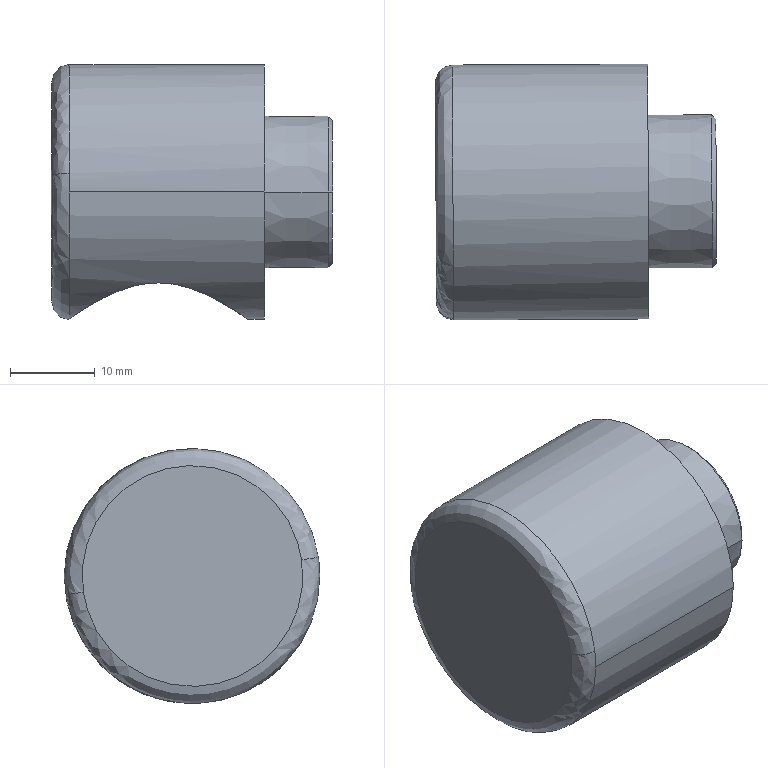Part | SolidWorks | features BaseBody 1 | 1 solid | 24 faces | box 33.093 x 30.1 x 30 mm | volume 10918 mm3 | cone 13 | spline 4 | cylinder 4 | plane 3 | commonest cylinder face diameters 16 x2 30 x2
STEP:
#1=CARTESIAN_POINT('',(688.091,25.759,6.001));
#2=VERTEX_POINT('',#1);
#3=CARTESIAN_POINT('',(687.979,51.477,2.182));
#4=VERTEX_POINT('',#3);
#5=CARTESIAN_POINT('',(688.091,25.759,6.001));
#6=CARTESIAN_POINT('',(688.107,21.94,-19.717));
#7=CARTESIAN_POINT('',(687.996,47.658,-23.536));
#8=CARTESIAN_POINT('',(687.979,51.477,2.182));
#9=(BOUNDED_CURVE()B_SPLINE_CURVE(3,(#5,#6,#7,#8),.UNSPECIFIED.,.F.,.F.)B_SPLINE_CURVE_WITH_KNOTS((4,4),(0.,1.),.UNSPECIFIED.)CURVE()GEOMETRIC_REPRESENTATION_ITEM()RATIONAL_B_SPLINE_CURVE((1.,0.3333,0.3333,1.))REPRESENTATION_ITEM(''));
#10=EDGE_CURVE('',#2,#4,#9,.T.);
#11=ORIENTED_EDGE('',*,*,#10,.T.);
#12=CARTESIAN_POINT('',(689.97,53.464,1.889));
#13=VERTEX_POINT('',#12);
#14=CARTESIAN_POINT('',(689.979,51.485,2.182));
#15=DIRECTION('',(0.0006392,-0.1469,-0.9892));
#16=DIRECTION('',(-0.004305,0.9891,-0.1469));
#17=AXIS2_PLACEMENT_3D('',#14,#15,#16);
#18=CIRCLE('',#17,2.);
#19=EDGE_CURVE('',#4,#13,#18,.T.);
#20=ORIENTED_EDGE('',*,*,#19,.T.);
#21=CARTESIAN_POINT('',(690.029,39.954,-10.849));
#22=VERTEX_POINT('',#21);
#23=CARTESIAN_POINT('',(690.035,38.626,4.092));
#24=DIRECTION('',(1.,0.004352,-0.000000001));
#25=DIRECTION('',(0.004352,-1.,0.));
#26=AXIS2_PLACEMENT_3D('',#23,#24,#25);
#27=CIRCLE('',#26,15.);
#28=EDGE_CURVE('',#22,#13,#27,.T.);
#29=ORIENTED_EDGE('',*,*,#28,.F.);
#30=CARTESIAN_POINT('',(690.041,37.299,-10.849));
#31=VERTEX_POINT('',#30);
#32=CARTESIAN_POINT('',(690.029,39.954,-10.849));
#33=CARTESIAN_POINT('',(689.974,39.511,-10.889));
#34=CARTESIAN_POINT('',(689.922,38.626,-10.924));
#35=CARTESIAN_POINT('',(689.982,37.741,-10.889));
#36=CARTESIAN_POINT('',(690.041,37.299,-10.849));
#37=B_SPLINE_CURVE_WITH_KNOTS('',3,(#32,#33,#34,#35,#36),.UNSPECIFIED.,.F.,.F.,(4,1,4),(0.,0.001328,0.002656),.UNSPECIFIED.);
#38=EDGE_CURVE('',#22,#31,#37,.T.);
#39=ORIENTED_EDGE('',*,*,#38,.T.);
#40=CARTESIAN_POINT('',(690.1,23.627,4.092));
#41=VERTEX_POINT('',#40);
#42=CARTESIAN_POINT('',(690.035,38.626,4.092));
#43=DIRECTION('',(1.,0.004352,-0.000000001));
#44=DIRECTION('',(0.004352,-1.,0.));
#45=AXIS2_PLACEMENT_3D('',#42,#43,#44);
#46=CIRCLE('',#45,15.);
#47=EDGE_CURVE('',#41,#31,#46,.T.);
#48=ORIENTED_EDGE('',*,*,#47,.F.);
#49=CARTESIAN_POINT('',(690.099,23.789,6.295));
#50=VERTEX_POINT('',#49);
#51=CARTESIAN_POINT('',(690.035,38.626,4.092));
#52=DIRECTION('',(1.,0.004352,-0.000000001));
#53=DIRECTION('',(0.004352,-1.,0.));
#54=AXIS2_PLACEMENT_3D('',#51,#52,#53);
#55=CIRCLE('',#54,15.);
#56=EDGE_CURVE('',#50,#41,#55,.T.);
#57=ORIENTED_EDGE('',*,*,#56,.F.);
#58=CARTESIAN_POINT('',(690.091,25.768,6.001));
#59=DIRECTION('',(-0.0006392,0.1469,0.9892));
#60=DIRECTION('',(0.004305,-0.9891,0.1469));
#61=AXIS2_PLACEMENT_3D('',#58,#59,#60);
#62=CIRCLE('',#61,2.);
#63=EDGE_CURVE('',#2,#50,#62,.T.);
#64=ORIENTED_EDGE('',*,*,#63,.F.);
#65=EDGE_LOOP('',(#11,#20,#29,#39,#48,#57,#64));
#66=FACE_OUTER_BOUND('',#65,.T.);
#67=CARTESIAN_POINT('',(687.979,51.477,2.182));
#68=CARTESIAN_POINT('',(687.996,47.658,-23.536));
#69=CARTESIAN_POINT('',(688.107,21.94,-19.717));
#70=CARTESIAN_POINT('',(688.091,25.759,6.001));
#71=CARTESIAN_POINT('',(687.974,52.636,2.01));
#72=CARTESIAN_POINT('',(687.992,48.473,-26.025));
#73=CARTESIAN_POINT('',(688.114,20.437,-21.863));
#74=CARTESIAN_POINT('',(688.096,24.6,6.173));
#75=CARTESIAN_POINT('',(688.799,53.459,1.889));
#76=CARTESIAN_POINT('',(688.818,49.053,-27.786));
#77=CARTESIAN_POINT('',(688.947,19.378,-23.38));
#78=CARTESIAN_POINT('',(688.928,23.784,6.295));
#79=CARTESIAN_POINT('',(689.97,53.464,1.889));
#80=CARTESIAN_POINT('',(689.989,49.058,-27.786));
#81=CARTESIAN_POINT('',(690.119,19.383,-23.38));
#82=CARTESIAN_POINT('',(690.099,23.789,6.295));
#83=(BOUNDED_SURFACE()B_SPLINE_SURFACE(3,3,((#67,#68,#69,#70),(#71,#72,#73,#74),(#75,#76,#77,#78),(#79,#80,#81,#82)),.UNSPECIFIED.,.F.,.F.,.F.)B_SPLINE_SURFACE_WITH_KNOTS((4,4),(4,4),(0.,1.),(0.,1.),.UNSPECIFIED.)GEOMETRIC_REPRESENTATION_ITEM()RATIONAL_B_SPLINE_SURFACE(((1.,0.3333,0.3333,1.),(0.8047,0.2682,0.2682,0.8047),(0.8047,0.2682,0.2682,0.8047),(1.,0.3333,0.3333,1.)))REPRESENTATION_ITEM('')SURFACE());
#84=ADVANCED_FACE('',(#66),#83,.T.);
#85=CARTESIAN_POINT('',(721.071,30.355,5.34));
#86=VERTEX_POINT('',#85);
#87=CARTESIAN_POINT('',(720.998,47.26,4.092));
#88=VERTEX_POINT('',#87);
#89=CARTESIAN_POINT('',(721.035,38.761,4.092));
#90=DIRECTION('',(-1.,-0.004352,0.000000001));
#91=DIRECTION('',(0.004305,-0.9891,0.1469));
#92=AXIS2_PLACEMENT_3D('',#89,#90,#91);
#93=CIRCLE('',#92,8.499);
#94=EDGE_CURVE('',#86,#88,#93,.T.);
#95=ORIENTED_EDGE('',*,*,#94,.F.);
#96=CARTESIAN_POINT('',(720.204,30.844,5.267));
#97=VERTEX_POINT('',#96);
#98=CARTESIAN_POINT('',(720.208,29.855,5.413));
#99=DIRECTION('',(-0.0006392,0.1469,0.9892));
#100=DIRECTION('',(0.004305,-0.9891,0.1469));
#101=AXIS2_PLACEMENT_3D('',#98,#99,#100);
#102=CIRCLE('',#101,1.);
#103=EDGE_CURVE('',#86,#97,#102,.T.);
#104=ORIENTED_EDGE('',*,*,#103,.T.);
#105=CARTESIAN_POINT('',(720.135,46.758,4.092));
#106=VERTEX_POINT('',#105);
#107=CARTESIAN_POINT('',(720.169,38.758,4.092));
#108=DIRECTION('',(-1.,-0.004352,0.000000001));
#109=DIRECTION('',(-0.004305,0.9891,-0.1469));
#110=AXIS2_PLACEMENT_3D('',#107,#108,#109);
#111=CIRCLE('',#110,8.);
#112=EDGE_CURVE('',#97,#106,#111,.T.);
#113=ORIENTED_EDGE('',*,*,#112,.T.);
#114=CARTESIAN_POINT('',(720.135,46.671,2.917));
#115=VERTEX_POINT('',#114);
#116=CARTESIAN_POINT('',(720.169,38.758,4.092));
#117=DIRECTION('',(-1.,-0.004352,0.000000001));
#118=DIRECTION('',(-0.004305,0.9891,-0.1469));
#119=AXIS2_PLACEMENT_3D('',#116,#117,#118);
#120=CIRCLE('',#119,8.);
#121=EDGE_CURVE('',#106,#115,#120,.T.);
#122=ORIENTED_EDGE('',*,*,#121,.T.);
#123=CARTESIAN_POINT('',(720.998,47.168,2.844));
#124=VERTEX_POINT('',#123);
#125=CARTESIAN_POINT('',(720.131,47.66,2.77));
#126=DIRECTION('',(0.0006392,-0.1469,-0.9892));
#127=DIRECTION('',(-0.004305,0.9891,-0.1469));
#128=AXIS2_PLACEMENT_3D('',#125,#126,#127);
#129=CIRCLE('',#128,1.);
#130=EDGE_CURVE('',#124,#115,#129,.T.);
#131=ORIENTED_EDGE('',*,*,#130,.F.);
#132=CARTESIAN_POINT('',(721.035,38.761,4.092));
#133=DIRECTION('',(-1.,-0.004352,0.000000001));
#134=DIRECTION('',(0.004305,-0.9891,0.1469));
#135=AXIS2_PLACEMENT_3D('',#132,#133,#134);
#136=CIRCLE('',#135,8.499);
#137=EDGE_CURVE('',#88,#124,#136,.T.);
#138=ORIENTED_EDGE('',*,*,#137,.F.);
#139=EDGE_LOOP('',(#95,#104,#113,#122,#131,#138));
#140=FACE_OUTER_BOUND('',#139,.T.);
#141=CARTESIAN_POINT('',(721.071,30.355,5.34));
#142=CARTESIAN_POINT('',(721.06,32.851,22.153));
#143=CARTESIAN_POINT('',(720.987,49.664,19.656));
#144=CARTESIAN_POINT('',(720.998,47.168,2.844));
#145=CARTESIAN_POINT('',(720.887,30.667,5.293));
#146=CARTESIAN_POINT('',(720.876,33.07,21.481));
#147=CARTESIAN_POINT('',(720.806,49.258,19.077));
#148=CARTESIAN_POINT('',(720.816,46.854,2.89));
#149=CARTESIAN_POINT('',(720.569,30.846,5.267));
#150=CARTESIAN_POINT('',(720.559,33.196,21.093));
#151=CARTESIAN_POINT('',(720.49,49.022,18.743));
#152=CARTESIAN_POINT('',(720.5,46.672,2.917));
#153=CARTESIAN_POINT('',(720.204,30.844,5.267));
#154=CARTESIAN_POINT('',(720.194,33.194,21.093));
#155=CARTESIAN_POINT('',(720.125,49.021,18.743));
#156=CARTESIAN_POINT('',(720.135,46.671,2.917));
#157=(BOUNDED_SURFACE()B_SPLINE_SURFACE(3,3,((#141,#142,#143,#144),(#145,#146,#147,#148),(#149,#150,#151,#152),(#153,#154,#155,#156)),.UNSPECIFIED.,.F.,.F.,.F.)B_SPLINE_SURFACE_WITH_KNOTS((4,4),(4,4),(0.,1.),(0.,1.),.UNSPECIFIED.)GEOMETRIC_REPRESENTATION_ITEM()RATIONAL_B_SPLINE_SURFACE(((1.,0.3333,0.3333,1.),(0.911,0.3037,0.3037,0.911),(0.911,0.3037,0.3037,0.911),(1.,0.3333,0.3333,1.)))REPRESENTATION_ITEM('')SURFACE());
#158=ADVANCED_FACE('',(#140),#157,.T.);
#159=CARTESIAN_POINT('',(713.1,23.727,4.092));
#160=VERTEX_POINT('',#159);
#161=CARTESIAN_POINT('',(712.969,53.726,4.092));
#162=VERTEX_POINT('',#161);
#163=CARTESIAN_POINT('',(713.035,38.727,4.092));
#164=DIRECTION('',(-1.,-0.004352,0.000000001));
#165=DIRECTION('',(0.004352,-1.,0.));
#166=AXIS2_PLACEMENT_3D('',#163,#164,#165);
#167=CIRCLE('',#166,15.);
#168=EDGE_CURVE('',#160,#162,#167,.T.);
#169=ORIENTED_EDGE('',*,*,#168,.T.);
#170=CARTESIAN_POINT('',(689.97,53.626,4.092));
#171=VERTEX_POINT('',#170);
#172=CARTESIAN_POINT('',(687.97,53.618,4.092));
#173=DIRECTION('',(-1.,-0.004352,0.000000001));
#174=VECTOR('',#173,1000.);
#175=LINE('',#172,#174);
#176=EDGE_CURVE('',#162,#171,#175,.T.);
#177=ORIENTED_EDGE('',*,*,#176,.T.);
#178=CARTESIAN_POINT('',(690.035,38.626,4.092));
#179=DIRECTION('',(1.,0.004352,-0.000000001));
#180=DIRECTION('',(0.004352,-1.,0.));
#181=AXIS2_PLACEMENT_3D('',#178,#179,#180);
#182=CIRCLE('',#181,15.);
#183=EDGE_CURVE('',#171,#50,#182,.T.);
#184=ORIENTED_EDGE('',*,*,#183,.T.);
#185=ORIENTED_EDGE('',*,*,#56,.T.);
#186=CARTESIAN_POINT('',(688.1,23.618,4.092));
#187=DIRECTION('',(-1.,-0.004352,0.000000001));
#188=VECTOR('',#187,1000.);
#189=LINE('',#186,#188);
#190=EDGE_CURVE('',#160,#41,#189,.T.);
#191=ORIENTED_EDGE('',*,*,#190,.F.);
#192=EDGE_LOOP('',(#169,#177,#184,#185,#191));
#193=FACE_OUTER_BOUND('',#192,.T.);
#194=CARTESIAN_POINT('',(688.035,38.618,4.092));
#195=DIRECTION('',(-1.,-0.004352,0.000000001));
#196=DIRECTION('',(0.004352,-1.,0.));
#197=AXIS2_PLACEMENT_3D('',#194,#195,#196);
#198=CYLINDRICAL_SURFACE('',#197,15.);
#199=ADVANCED_FACE('',(#193),#198,.T.);
#200=CARTESIAN_POINT('',(720.574,29.761,4.092));
#201=VERTEX_POINT('',#200);
#202=CARTESIAN_POINT('',(720.495,47.758,4.092));
#203=VERTEX_POINT('',#202);
#204=CARTESIAN_POINT('',(720.535,38.759,4.092));
#205=DIRECTION('',(-1.,-0.004352,0.000000001));
#206=DIRECTION('',(-0.004305,0.9891,-0.1469));
#207=AXIS2_PLACEMENT_3D('',#204,#205,#206);
#208=CIRCLE('',#207,8.999);
#209=EDGE_CURVE('',#201,#203,#208,.T.);
#210=ORIENTED_EDGE('',*,*,#209,.T.);
#211=CARTESIAN_POINT('',(712.995,47.726,4.092));
#212=VERTEX_POINT('',#211);
#213=CARTESIAN_POINT('',(712.995,47.726,4.092));
#214=DIRECTION('',(-1.,-0.004178,0.000000001));
#215=VECTOR('',#214,1000.);
#216=LINE('',#213,#215);
#217=EDGE_CURVE('',#203,#212,#216,.T.);
#218=ORIENTED_EDGE('',*,*,#217,.T.);
#219=CARTESIAN_POINT('',(713.074,29.727,4.092));
#220=VERTEX_POINT('',#219);
#221=CARTESIAN_POINT('',(713.035,38.727,4.092));
#222=DIRECTION('',(-1.,-0.004352,0.000000001));
#223=DIRECTION('',(0.004352,-1.,0.));
#224=AXIS2_PLACEMENT_3D('',#221,#222,#223);
#225=CIRCLE('',#224,9.);
#226=EDGE_CURVE('',#220,#212,#225,.T.);
#227=ORIENTED_EDGE('',*,*,#226,.F.);
#228=CARTESIAN_POINT('',(713.074,29.727,4.092));
#229=DIRECTION('',(-1.,-0.004527,0.000000001));
#230=VECTOR('',#229,1000.);
#231=LINE('',#228,#230);
#232=EDGE_CURVE('',#201,#220,#231,.T.);
#233=ORIENTED_EDGE('',*,*,#232,.F.);
#234=EDGE_LOOP('',(#210,#218,#227,#233));
#235=FACE_OUTER_BOUND('',#234,.T.);
#236=CARTESIAN_POINT('',(713.035,38.727,4.092));
#237=DIRECTION('',(-1.,-0.004352,0.000000001));
#238=DIRECTION('',(0.004352,-1.,0.));
#239=AXIS2_PLACEMENT_3D('',#236,#237,#238);
#240=CONICAL_SURFACE('',#239,9.,0.0001745);
#241=ADVANCED_FACE('',(#235),#240,.T.);
#242=CARTESIAN_POINT('',(700.535,28.172,-6.059));
#243=VERTEX_POINT('',#242);
#244=CARTESIAN_POINT('',(700.535,49.172,-6.059));
#245=VERTEX_POINT('',#244);
#246=CARTESIAN_POINT('',(700.535,38.672,-6.059));
#247=DIRECTION('',(-0.000000001,0.000000003,-1.));
#248=DIRECTION('',(0.,1.,0.000000003));
#249=AXIS2_PLACEMENT_3D('',#246,#247,#248);
#250=CIRCLE('',#249,10.5);
#251=EDGE_CURVE('',#243,#245,#250,.T.);
#252=ORIENTED_EDGE('',*,*,#251,.F.);
#253=CARTESIAN_POINT('',(700.535,28.163,-6.611));
#254=VERTEX_POINT('',#253);
#255=CARTESIAN_POINT('',(700.535,28.087,-10.936));
#256=DIRECTION('',(-0.000000001,-0.01745,-0.9998));
#257=VECTOR('',#256,1000.);
#258=LINE('',#255,#257);
#259=EDGE_CURVE('',#243,#254,#258,.T.);
#260=ORIENTED_EDGE('',*,*,#259,.T.);
#261=CARTESIAN_POINT('',(690.041,37.299,-10.849));
#262=CARTESIAN_POINT('',(690.128,36.64,-10.791));
#263=CARTESIAN_POINT('',(690.275,36.006,-10.691));
#264=CARTESIAN_POINT('',(690.577,35.091,-10.488));
#265=CARTESIAN_POINT('',(690.691,34.791,-10.412));
#266=CARTESIAN_POINT('',(690.947,34.204,-10.244));
#267=CARTESIAN_POINT('',(691.089,33.915,-10.151));
#268=CARTESIAN_POINT('',(691.544,33.085,-9.857));
#269=CARTESIAN_POINT('',(691.891,32.57,-9.638));
#270=CARTESIAN_POINT('',(692.474,31.849,-9.287));
#271=CARTESIAN_POINT('',(692.68,31.616,-9.166));
#272=CARTESIAN_POINT('',(693.108,31.173,-8.92));
#273=CARTESIAN_POINT('',(693.33,30.963,-8.796));
#274=CARTESIAN_POINT('',(694.02,30.362,-8.424));
#275=CARTESIAN_POINT('',(694.513,30.004,-8.175));
#276=CARTESIAN_POINT('',(695.307,29.526,-7.816));
#277=CARTESIAN_POINT('',(695.581,29.376,-7.699));
#278=CARTESIAN_POINT('',(696.141,29.103,-7.477));
#279=CARTESIAN_POINT('',(696.427,28.979,-7.372));
#280=CARTESIAN_POINT('',(697.014,28.754,-7.176));
#281=CARTESIAN_POINT('',(697.314,28.654,-7.086));
#282=CARTESIAN_POINT('',(697.931,28.48,-6.925));
#283=CARTESIAN_POINT('',(698.249,28.405,-6.853));
#284=CARTESIAN_POINT('',(699.213,28.224,-6.678));
#285=CARTESIAN_POINT('',(699.867,28.162,-6.614));
#286=CARTESIAN_POINT('',(700.535,28.163,-6.611));
#287=B_SPLINE_CURVE_WITH_KNOTS('',3,(#261,#262,#263,#264,#265,#266,#267,#268,#269,#270,#271,#272,#273,#274,#275,#276,#277,#278,#279,#280,#281,#282,#283,#284,#285,#286),.UNSPECIFIED.,.F.,.F.,(4,2,2,2,2,2,2,2,2,2,2,2,4),(-0.05002,-0.04806,-0.04707,-0.04609,-0.04412,-0.04313,-0.04215,-0.04018,-0.0392,-0.03821,-0.03723,-0.03624,-0.03427),.UNSPECIFIED.);
#288=EDGE_CURVE('',#31,#254,#287,.T.);
#289=ORIENTED_EDGE('',*,*,#288,.F.);
#290=ORIENTED_EDGE('',*,*,#38,.F.);
#291=CARTESIAN_POINT('',(700.535,49.182,-6.611));
#292=VERTEX_POINT('',#291);
#293=CARTESIAN_POINT('',(700.535,49.182,-6.611));
#294=CARTESIAN_POINT('',(699.863,49.182,-6.608));
#295=CARTESIAN_POINT('',(699.206,49.119,-6.668));
#296=CARTESIAN_POINT('',(697.926,48.879,-6.891));
#297=CARTESIAN_POINT('',(697.295,48.698,-7.057));
#298=CARTESIAN_POINT('',(696.11,48.242,-7.447));
#299=CARTESIAN_POINT('',(695.549,47.966,-7.672));
#300=CARTESIAN_POINT('',(694.482,47.319,-8.153));
#301=CARTESIAN_POINT('',(693.985,46.954,-8.405));
#302=CARTESIAN_POINT('',(693.293,46.347,-8.779));
#303=CARTESIAN_POINT('',(693.071,46.135,-8.904));
#304=CARTESIAN_POINT('',(692.645,45.688,-9.151));
#305=CARTESIAN_POINT('',(692.439,45.453,-9.273));
#306=CARTESIAN_POINT('',(691.855,44.723,-9.628));
#307=CARTESIAN_POINT('',(691.511,44.205,-9.847));
#308=CARTESIAN_POINT('',(691.062,43.376,-10.141));
#309=CARTESIAN_POINT('',(690.924,43.091,-10.233));
#310=CARTESIAN_POINT('',(690.672,42.503,-10.403));
#311=CARTESIAN_POINT('',(690.557,42.198,-10.481));
#312=CARTESIAN_POINT('',(690.255,41.262,-10.689));
#313=CARTESIAN_POINT('',(690.111,40.618,-10.79));
#314=CARTESIAN_POINT('',(690.029,39.954,-10.849));
#315=B_SPLINE_CURVE_WITH_KNOTS('',3,(#293,#294,#295,#296,#297,#298,#299,#300,#301,#302,#303,#304,#305,#306,#307,#308,#309,#310,#311,#312,#313,#314),.UNSPECIFIED.,.F.,.F.,(4,2,2,2,2,2,2,2,2,2,4),(-0.0000449,0.001935,0.003914,0.005894,0.007873,0.008863,0.009853,0.01183,0.01282,0.01381,0.01579),.UNSPECIFIED.);
#316=EDGE_CURVE('',#292,#22,#315,.T.);
#317=ORIENTED_EDGE('',*,*,#316,.F.);
#318=CARTESIAN_POINT('',(700.535,49.257,-10.936));
#319=DIRECTION('',(-0.000000001,0.01745,-0.9998));
#320=VECTOR('',#319,1000.);
#321=LINE('',#318,#320);
#322=EDGE_CURVE('',#245,#292,#321,.T.);
#323=ORIENTED_EDGE('',*,*,#322,.F.);
#324=EDGE_LOOP('',(#252,#260,#289,#290,#317,#323));
#325=FACE_OUTER_BOUND('',#324,.T.);
#326=CARTESIAN_POINT('',(700.535,38.672,-10.936));
#327=DIRECTION('',(-0.000000001,0.000000003,-1.));
#328=DIRECTION('',(0.,1.,0.000000003));
#329=AXIS2_PLACEMENT_3D('',#326,#327,#328);
#330=CONICAL_SURFACE('',#329,10.585,0.01745);
#331=ADVANCED_FACE('',(#325),#330,.F.);
#332=CARTESIAN_POINT('',(721.072,30.263,4.092));
#333=VERTEX_POINT('',#332);
#334=CARTESIAN_POINT('',(721.035,38.761,4.092));
#335=DIRECTION('',(-1.,-0.004352,0.000000001));
#336=DIRECTION('',(0.004305,-0.9891,0.1469));
#337=AXIS2_PLACEMENT_3D('',#334,#335,#336);
#338=CIRCLE('',#337,8.499);
#339=EDGE_CURVE('',#333,#86,#338,.T.);
#340=ORIENTED_EDGE('',*,*,#339,.T.);
#341=ORIENTED_EDGE('',*,*,#94,.T.);
#342=CARTESIAN_POINT('',(720.495,47.758,4.092));
#343=DIRECTION('',(-0.7101,0.7041,0.000000001));
#344=VECTOR('',#343,1000.);
#345=LINE('',#342,#344);
#346=EDGE_CURVE('',#88,#203,#345,.T.);
#347=ORIENTED_EDGE('',*,*,#346,.T.);
#348=ORIENTED_EDGE('',*,*,#209,.F.);
#349=CARTESIAN_POINT('',(720.574,29.761,4.092));
#350=DIRECTION('',(-0.704,-0.7102,0.000000001));
#351=VECTOR('',#350,1000.);
#352=LINE('',#349,#351);
#353=EDGE_CURVE('',#333,#201,#352,.T.);
#354=ORIENTED_EDGE('',*,*,#353,.F.);
#355=EDGE_LOOP('',(#340,#341,#347,#348,#354));
#356=FACE_OUTER_BOUND('',#355,.T.);
#357=CARTESIAN_POINT('',(720.535,38.759,4.092));
#358=DIRECTION('',(-1.,-0.004352,0.000000001));
#359=DIRECTION('',(0.004352,-1.,0.));
#360=AXIS2_PLACEMENT_3D('',#357,#358,#359);
#361=CONICAL_SURFACE('',#360,8.999,0.7855);
#362=ADVANCED_FACE('',(#356),#361,.T.);
#363=CARTESIAN_POINT('',(700.535,29.02,-0.05868));
#364=VERTEX_POINT('',#363);
#365=CARTESIAN_POINT('',(700.535,48.324,-0.05868));
#366=VERTEX_POINT('',#365);
#367=CARTESIAN_POINT('',(700.535,38.672,-0.05868));
#368=DIRECTION('',(-0.000000001,0.000000003,-1.));
#369=DIRECTION('',(-0.004352,1.,0.000000003));
#370=AXIS2_PLACEMENT_3D('',#367,#368,#369);
#371=CIRCLE('',#370,9.652);
#372=EDGE_CURVE('',#364,#366,#371,.T.);
#373=ORIENTED_EDGE('',*,*,#372,.F.);
#374=CARTESIAN_POINT('',(700.535,28.91,-6.059));
#375=VERTEX_POINT('',#374);
#376=CARTESIAN_POINT('',(700.535,28.91,-6.059));
#377=DIRECTION('',(-0.000000001,-0.01826,-0.9998));
#378=VECTOR('',#377,1000.);
#379=LINE('',#376,#378);
#380=EDGE_CURVE('',#364,#375,#379,.T.);
#381=ORIENTED_EDGE('',*,*,#380,.T.);
#382=CARTESIAN_POINT('',(700.535,48.434,-6.059));
#383=VERTEX_POINT('',#382);
#384=CARTESIAN_POINT('',(700.535,38.672,-6.059));
#385=DIRECTION('',(-0.000000001,0.000000003,-1.));
#386=DIRECTION('',(0.,1.,0.000000003));
#387=AXIS2_PLACEMENT_3D('',#384,#385,#386);
#388=CIRCLE('',#387,9.762);
#389=EDGE_CURVE('',#375,#383,#388,.T.);
#390=ORIENTED_EDGE('',*,*,#389,.T.);
#391=CARTESIAN_POINT('',(700.535,48.434,-6.059));
#392=DIRECTION('',(-0.000000001,0.01826,-0.9998));
#393=VECTOR('',#392,1000.);
#394=LINE('',#391,#393);
#395=EDGE_CURVE('',#366,#383,#394,.T.);
#396=ORIENTED_EDGE('',*,*,#395,.F.);
#397=EDGE_LOOP('',(#373,#381,#390,#396));
#398=FACE_OUTER_BOUND('',#397,.T.);
#399=CARTESIAN_POINT('',(700.535,38.672,-6.059));
#400=DIRECTION('',(-0.000000001,0.000000003,-1.));
#401=DIRECTION('',(0.,1.,0.000000003));
#402=AXIS2_PLACEMENT_3D('',#399,#400,#401);
#403=CONICAL_SURFACE('',#402,9.762,0.01826);
#404=ADVANCED_FACE('',(#398),#403,.F.);
#405=ORIENTED_EDGE('',*,*,#121,.F.);
#406=CARTESIAN_POINT('',(705.774,46.695,4.092));
#407=VERTEX_POINT('',#406);
#408=CARTESIAN_POINT('',(710.5,46.716,4.092));
#409=DIRECTION('',(-1.,-0.004352,0.000000001));
#410=VECTOR('',#409,1000.);
#411=LINE('',#408,#410);
#412=EDGE_CURVE('',#106,#407,#411,.T.);
#413=ORIENTED_EDGE('',*,*,#412,.T.);
#414=CARTESIAN_POINT('',(707.316,45.541,-0.05868));
#415=VERTEX_POINT('',#414);
#416=CARTESIAN_POINT('',(707.316,45.541,-0.05868));
#417=CARTESIAN_POINT('',(707.129,45.719,0.2354));
#418=CARTESIAN_POINT('',(706.947,45.877,0.5401));
#419=CARTESIAN_POINT('',(706.601,46.156,1.175));
#420=CARTESIAN_POINT('',(706.438,46.277,1.506));
#421=CARTESIAN_POINT('',(706.149,46.479,2.202));
#422=CARTESIAN_POINT('',(706.023,46.559,2.568));
#423=CARTESIAN_POINT('',(705.841,46.667,3.323));
#424=CARTESIAN_POINT('',(705.786,46.695,3.705));
#425=CARTESIAN_POINT('',(705.774,46.695,4.092));
#426=B_SPLINE_CURVE_WITH_KNOTS('',3,(#416,#417,#418,#419,#420,#421,#422,#423,#424,#425),.UNSPECIFIED.,.F.,.F.,(4,2,2,2,4),(-0.003444,-0.002286,-0.001128,0.00002938,0.001187),.UNSPECIFIED.);
#427=EDGE_CURVE('',#415,#407,#426,.T.);
#428=ORIENTED_EDGE('',*,*,#427,.F.);
#429=CARTESIAN_POINT('',(707.376,31.863,-0.05868));
#430=VERTEX_POINT('',#429);
#431=CARTESIAN_POINT('',(707.316,45.541,-0.05868));
#432=CARTESIAN_POINT('',(707.67,45.206,-0.6135));
#433=CARTESIAN_POINT('',(708.028,44.813,-1.115));
#434=CARTESIAN_POINT('',(708.711,43.901,-2.028));
#435=CARTESIAN_POINT('',(709.039,43.374,-2.443));
#436=CARTESIAN_POINT('',(709.458,42.503,-2.96));
#437=CARTESIAN_POINT('',(709.586,42.199,-3.117));
#438=CARTESIAN_POINT('',(709.816,41.558,-3.393));
#439=CARTESIAN_POINT('',(709.917,41.22,-3.514));
#440=CARTESIAN_POINT('',(710.08,40.533,-3.707));
#441=CARTESIAN_POINT('',(710.144,40.18,-3.781));
#442=CARTESIAN_POINT('',(710.232,39.457,-3.882));
#443=CARTESIAN_POINT('',(710.255,39.085,-3.908));
#444=CARTESIAN_POINT('',(710.259,38.354,-3.909));
#445=CARTESIAN_POINT('',(710.24,37.99,-3.884));
#446=CARTESIAN_POINT('',(710.16,37.265,-3.785));
#447=CARTESIAN_POINT('',(710.098,36.905,-3.709));
#448=CARTESIAN_POINT('',(709.941,36.215,-3.517));
#449=CARTESIAN_POINT('',(709.845,35.882,-3.399));
#450=CARTESIAN_POINT('',(709.621,35.235,-3.122));
#451=CARTESIAN_POINT('',(709.494,34.925,-2.964));
#452=CARTESIAN_POINT('',(709.219,34.342,-2.619));
#453=CARTESIAN_POINT('',(709.072,34.066,-2.431));
#454=CARTESIAN_POINT('',(708.759,33.543,-2.026));
#455=CARTESIAN_POINT('',(708.594,33.294,-1.808));
#456=CARTESIAN_POINT('',(708.083,32.598,-1.117));
#457=CARTESIAN_POINT('',(707.727,32.201,-0.6138));
#458=CARTESIAN_POINT('',(707.376,31.863,-0.05868));
#459=B_SPLINE_CURVE_WITH_KNOTS('',3,(#431,#432,#433,#434,#435,#436,#437,#438,#439,#440,#441,#442,#443,#444,#445,#446,#447,#448,#449,#450,#451,#452,#453,#454,#455,#456,#457,#458),.UNSPECIFIED.,.F.,.F.,(4,2,2,2,2,2,2,2,2,2,2,2,2,4),(0.,0.002187,0.004374,0.005468,0.006562,0.007655,0.008749,0.009842,0.01094,0.01203,0.01312,0.01422,0.01531,0.0175),.UNSPECIFIED.);
#460=EDGE_CURVE('',#415,#430,#459,.T.);
#461=ORIENTED_EDGE('',*,*,#460,.T.);
#462=CARTESIAN_POINT('',(705.844,30.695,4.092));
#463=VERTEX_POINT('',#462);
#464=CARTESIAN_POINT('',(705.844,30.695,4.092));
#465=CARTESIAN_POINT('',(705.85,30.695,3.897));
#466=CARTESIAN_POINT('',(705.867,30.703,3.7));
#467=CARTESIAN_POINT('',(705.921,30.731,3.314));
#468=CARTESIAN_POINT('',(705.958,30.752,3.124));
#469=CARTESIAN_POINT('',(706.093,30.835,2.562));
#470=CARTESIAN_POINT('',(706.219,30.916,2.196));
#471=CARTESIAN_POINT('',(706.506,31.12,1.502));
#472=CARTESIAN_POINT('',(706.667,31.242,1.173));
#473=CARTESIAN_POINT('',(707.009,31.524,0.5394));
#474=CARTESIAN_POINT('',(707.19,31.684,0.2352));
#475=CARTESIAN_POINT('',(707.376,31.863,-0.05868));
#476=B_SPLINE_CURVE_WITH_KNOTS('',3,(#464,#465,#466,#467,#468,#469,#470,#471,#472,#473,#474,#475),.UNSPECIFIED.,.F.,.F.,(4,2,2,2,2,4),(0.005549,0.006131,0.006713,0.007877,0.009041,0.0102),.UNSPECIFIED.);
#477=EDGE_CURVE('',#463,#430,#476,.T.);
#478=ORIENTED_EDGE('',*,*,#477,.F.);
#479=CARTESIAN_POINT('',(720.204,30.758,4.092));
#480=VERTEX_POINT('',#479);
#481=CARTESIAN_POINT('',(710.569,30.716,4.092));
#482=DIRECTION('',(-1.,-0.004352,0.000000001));
#483=VECTOR('',#482,1000.);
#484=LINE('',#481,#483);
#485=EDGE_CURVE('',#480,#463,#484,.T.);
#486=ORIENTED_EDGE('',*,*,#485,.F.);
#487=CARTESIAN_POINT('',(720.169,38.758,4.092));
#488=DIRECTION('',(-1.,-0.004352,0.000000001));
#489=DIRECTION('',(-0.004305,0.9891,-0.1469));
#490=AXIS2_PLACEMENT_3D('',#487,#488,#489);
#491=CIRCLE('',#490,8.);
#492=EDGE_CURVE('',#115,#480,#491,.T.);
#493=ORIENTED_EDGE('',*,*,#492,.F.);
#494=EDGE_LOOP('',(#405,#413,#428,#461,#478,#486,#493));
#495=FACE_OUTER_BOUND('',#494,.T.);
#496=CARTESIAN_POINT('',(710.535,38.716,4.092));
#497=DIRECTION('',(-1.,-0.004352,0.000000001));
#498=DIRECTION('',(0.004352,-1.,0.));
#499=AXIS2_PLACEMENT_3D('',#496,#497,#498);
#500=CYLINDRICAL_SURFACE('',#499,8.);
#501=ADVANCED_FACE('',(#495),#500,.F.);
#502=CARTESIAN_POINT('',(700.535,29.172,8.941));
#503=VERTEX_POINT('',#502);
#504=CARTESIAN_POINT('',(700.535,48.172,8.941));
#505=VERTEX_POINT('',#504);
#506=CARTESIAN_POINT('',(700.535,38.672,8.941));
#507=DIRECTION('',(-0.000000001,0.000000003,-1.));
#508=DIRECTION('',(-0.004352,1.,0.000000003));
#509=AXIS2_PLACEMENT_3D('',#506,#507,#508);
#510=CIRCLE('',#509,9.5);
#511=EDGE_CURVE('',#503,#505,#510,.T.);
#512=ORIENTED_EDGE('',*,*,#511,.F.);
#513=CARTESIAN_POINT('',(700.535,29.02,-0.05868));
#514=DIRECTION('',(-0.000000001,-0.01692,-0.9999));
#515=VECTOR('',#514,1000.);
#516=LINE('',#513,#515);
#517=EDGE_CURVE('',#503,#364,#516,.T.);
#518=ORIENTED_EDGE('',*,*,#517,.T.);
#519=ORIENTED_EDGE('',*,*,#372,.T.);
#520=CARTESIAN_POINT('',(700.535,48.324,-0.05868));
#521=DIRECTION('',(-0.000000001,0.01692,-0.9999));
#522=VECTOR('',#521,1000.);
#523=LINE('',#520,#522);
#524=EDGE_CURVE('',#505,#366,#523,.T.);
#525=ORIENTED_EDGE('',*,*,#524,.F.);
#526=EDGE_LOOP('',(#512,#518,#519,#525));
#527=FACE_OUTER_BOUND('',#526,.T.);
#528=CARTESIAN_POINT('',(700.535,38.672,-0.05868));
#529=DIRECTION('',(-0.000000001,0.000000003,-1.));
#530=DIRECTION('',(0.,1.,0.000000003));
#531=AXIS2_PLACEMENT_3D('',#528,#529,#530);
#532=CONICAL_SURFACE('',#531,9.652,0.01692);
#533=ADVANCED_FACE('',(#527),#532,.F.);
#534=CARTESIAN_POINT('',(707.562,45.065,8.941));
#535=VERTEX_POINT('',#534);
#536=CARTESIAN_POINT('',(700.535,38.672,8.941));
#537=DIRECTION('',(-0.000000001,0.000000003,-1.));
#538=DIRECTION('',(-0.004352,1.,0.000000003));
#539=AXIS2_PLACEMENT_3D('',#536,#537,#538);
#540=CIRCLE('',#539,9.5);
#541=EDGE_CURVE('',#505,#535,#540,.T.);
#542=ORIENTED_EDGE('',*,*,#541,.F.);
#543=ORIENTED_EDGE('',*,*,#524,.T.);
#544=CARTESIAN_POINT('',(700.535,38.672,-0.05868));
#545=DIRECTION('',(-0.000000001,0.000000003,-1.));
#546=DIRECTION('',(-0.004352,1.,0.000000003));
#547=AXIS2_PLACEMENT_3D('',#544,#545,#546);
#548=CIRCLE('',#547,9.652);
#549=EDGE_CURVE('',#366,#415,#548,.T.);
#550=ORIENTED_EDGE('',*,*,#549,.T.);
#551=ORIENTED_EDGE('',*,*,#427,.T.);
#552=CARTESIAN_POINT('',(705.774,46.695,4.092));
#553=CARTESIAN_POINT('',(705.767,46.695,4.322));
#554=CARTESIAN_POINT('',(705.775,46.685,4.557));
#555=CARTESIAN_POINT('',(705.822,46.645,5.021));
#556=CARTESIAN_POINT('',(705.86,46.615,5.247));
#557=CARTESIAN_POINT('',(705.961,46.537,5.692));
#558=CARTESIAN_POINT('',(706.023,46.49,5.91));
#559=CARTESIAN_POINT('',(706.167,46.378,6.339));
#560=CARTESIAN_POINT('',(706.248,46.313,6.549));
#561=CARTESIAN_POINT('',(706.51,46.1,7.158));
#562=CARTESIAN_POINT('',(706.708,45.93,7.539));
#563=CARTESIAN_POINT('',(707.124,45.538,8.266));
#564=CARTESIAN_POINT('',(707.343,45.314,8.613));
#565=CARTESIAN_POINT('',(707.562,45.065,8.941));
#566=B_SPLINE_CURVE_WITH_KNOTS('',3,(#552,#553,#554,#555,#556,#557,#558,#559,#560,#561,#562,#563,#564,#565),.UNSPECIFIED.,.F.,.F.,(4,2,2,2,2,2,4),(0.001187,0.001878,0.002569,0.003261,0.003952,0.005334,0.006717),.UNSPECIFIED.);
#567=EDGE_CURVE('',#407,#535,#566,.T.);
#568=ORIENTED_EDGE('',*,*,#567,.T.);
#569=EDGE_LOOP('',(#542,#543,#550,#551,#568));
#570=FACE_OUTER_BOUND('',#569,.T.);
#571=CARTESIAN_POINT('',(700.535,38.672,-0.05868));
#572=DIRECTION('',(-0.000000001,0.000000003,-1.));
#573=DIRECTION('',(0.,1.,0.000000003));
#574=AXIS2_PLACEMENT_3D('',#571,#572,#573);
#575=CONICAL_SURFACE('',#574,9.652,0.01692);
#576=ADVANCED_FACE('',(#570),#575,.F.);
#577=CARTESIAN_POINT('',(700.535,38.672,14.649));
#578=VERTEX_POINT('',#577);
#579=CARTESIAN_POINT('',(700.535,48.172,8.941));
#580=DIRECTION('',(0.,0.8572,-0.515));
#581=VECTOR('',#580,1000.);
#582=LINE('',#579,#581);
#583=EDGE_CURVE('',#578,#505,#582,.T.);
#584=ORIENTED_EDGE('',*,*,#583,.F.);
#585=CARTESIAN_POINT('',(700.535,29.172,8.941));
#586=DIRECTION('',(0.,-0.8572,-0.515));
#587=VECTOR('',#586,1000.);
#588=LINE('',#585,#587);
#589=EDGE_CURVE('',#578,#503,#588,.T.);
#590=ORIENTED_EDGE('',*,*,#589,.T.);
#591=ORIENTED_EDGE('',*,*,#511,.T.);
#592=EDGE_LOOP('',(#584,#590,#591));
#593=FACE_OUTER_BOUND('',#592,.T.);
#594=CARTESIAN_POINT('',(700.535,38.672,8.941));
#595=DIRECTION('',(-0.000000001,0.000000003,-1.));
#596=DIRECTION('',(0.,1.,0.000000003));
#597=AXIS2_PLACEMENT_3D('',#594,#595,#596);
#598=CONICAL_SURFACE('',#597,9.5,1.03);
#599=ADVANCED_FACE('',(#593),#598,.F.);
#600=ORIENTED_EDGE('',*,*,#176,.F.);
#601=CARTESIAN_POINT('',(713.035,38.727,4.092));
#602=DIRECTION('',(-1.,-0.004352,0.000000001));
#603=DIRECTION('',(0.004352,-1.,0.));
#604=AXIS2_PLACEMENT_3D('',#601,#602,#603);
#605=CIRCLE('',#604,15.);
#606=EDGE_CURVE('',#162,#160,#605,.T.);
#607=ORIENTED_EDGE('',*,*,#606,.T.);
#608=ORIENTED_EDGE('',*,*,#190,.T.);
#609=ORIENTED_EDGE('',*,*,#47,.T.);
#610=ORIENTED_EDGE('',*,*,#288,.T.);
#611=CARTESIAN_POINT('',(700.535,28.163,-6.611));
#612=CARTESIAN_POINT('',(701.26,28.163,-6.608));
#613=CARTESIAN_POINT('',(701.968,28.236,-6.678));
#614=CARTESIAN_POINT('',(703.,28.445,-6.872));
#615=CARTESIAN_POINT('',(703.342,28.532,-6.951));
#616=CARTESIAN_POINT('',(704.01,28.738,-7.135));
#617=CARTESIAN_POINT('',(704.333,28.855,-7.237));
#618=CARTESIAN_POINT('',(704.962,29.118,-7.458));
#619=CARTESIAN_POINT('',(705.268,29.264,-7.576));
#620=CARTESIAN_POINT('',(705.862,29.582,-7.824));
#621=CARTESIAN_POINT('',(706.152,29.755,-7.954));
#622=CARTESIAN_POINT('',(706.988,30.312,-8.352));
#623=CARTESIAN_POINT('',(707.502,30.729,-8.625));
#624=CARTESIAN_POINT('',(708.45,31.659,-9.161));
#625=CARTESIAN_POINT('',(708.888,32.178,-9.426));
#626=CARTESIAN_POINT('',(709.65,33.285,-9.905));
#627=CARTESIAN_POINT('',(709.98,33.875,-10.122));
#628=CARTESIAN_POINT('',(710.392,34.825,-10.399));
#629=CARTESIAN_POINT('',(710.516,35.155,-10.484));
#630=CARTESIAN_POINT('',(710.731,35.828,-10.632));
#631=CARTESIAN_POINT('',(710.822,36.17,-10.695));
#632=CARTESIAN_POINT('',(710.968,36.863,-10.797));
#633=CARTESIAN_POINT('',(711.023,37.214,-10.837));
#634=CARTESIAN_POINT('',(711.099,37.927,-10.892));
#635=CARTESIAN_POINT('',(711.119,38.29,-10.907));
#636=CARTESIAN_POINT('',(711.121,39.371,-10.911));
#637=CARTESIAN_POINT('',(711.049,40.081,-10.863));
#638=CARTESIAN_POINT('',(710.833,41.129,-10.717));
#639=CARTESIAN_POINT('',(710.743,41.477,-10.656));
#640=CARTESIAN_POINT('',(710.531,42.149,-10.514));
#641=CARTESIAN_POINT('',(710.409,42.477,-10.433));
#642=CARTESIAN_POINT('',(709.999,43.433,-10.162));
#643=CARTESIAN_POINT('',(709.662,44.042,-9.943));
#644=CARTESIAN_POINT('',(708.895,45.158,-9.465));
#645=CARTESIAN_POINT('',(708.465,45.67,-9.205));
#646=CARTESIAN_POINT('',(707.509,46.611,-8.666));
#647=CARTESIAN_POINT('',(706.992,47.03,-8.392));
#648=CARTESIAN_POINT('',(706.163,47.582,-7.996));
#649=CARTESIAN_POINT('',(705.878,47.754,-7.866));
#650=CARTESIAN_POINT('',(705.285,48.073,-7.616));
#651=CARTESIAN_POINT('',(704.976,48.22,-7.494));
#652=CARTESIAN_POINT('',(704.028,48.618,-7.156));
#653=CARTESIAN_POINT('',(703.369,48.823,-6.965));
#654=CARTESIAN_POINT('',(702.33,49.036,-6.76));
#655=CARTESIAN_POINT('',(701.973,49.091,-6.706));
#656=CARTESIAN_POINT('',(701.258,49.163,-6.632));
#657=CARTESIAN_POINT('',(700.898,49.182,-6.613));
#658=CARTESIAN_POINT('',(700.535,49.182,-6.611));
#659=B_SPLINE_CURVE_WITH_KNOTS('',3,(#611,#612,#613,#614,#615,#616,#617,#618,#619,#620,#621,#622,#623,#624,#625,#626,#627,#628,#629,#630,#631,#632,#633,#634,#635,#636,#637,#638,#639,#640,#641,#642,#643,#644,#645,#646,#647,#648,#649,#650,#651,#652,#653,#654,#655,#656,#657,#658),.UNSPECIFIED.,.F.,.F.,(4,2,2,2,2,2,2,2,2,2,2,2,2,2,2,2,2,2,2,2,2,2,2,4),(-0.03427,-0.03213,-0.03107,-0.03,-0.02893,-0.02786,-0.02572,-0.02358,-0.02144,-0.02037,-0.0193,-0.01823,-0.01716,-0.01502,-0.01395,-0.01288,-0.01074,-0.008602,-0.006463,-0.005393,-0.004324,-0.002184,-0.001115,-0.0000449),.UNSPECIFIED.);
#660=EDGE_CURVE('',#254,#292,#659,.T.);
#661=ORIENTED_EDGE('',*,*,#660,.T.);
#662=ORIENTED_EDGE('',*,*,#316,.T.);
#663=ORIENTED_EDGE('',*,*,#28,.T.);
#664=CARTESIAN_POINT('',(690.035,38.626,4.092));
#665=DIRECTION('',(1.,0.004352,-0.000000001));
#666=DIRECTION('',(0.004352,-1.,0.));
#667=AXIS2_PLACEMENT_3D('',#664,#665,#666);
#668=CIRCLE('',#667,15.);
#669=EDGE_CURVE('',#13,#171,#668,.T.);
#670=ORIENTED_EDGE('',*,*,#669,.T.);
#671=EDGE_LOOP('',(#600,#607,#608,#609,#610,#661,#662,#663,#670));
#672=FACE_OUTER_BOUND('',#671,.T.);
#673=CARTESIAN_POINT('',(688.035,38.618,4.092));
#674=DIRECTION('',(-1.,-0.004352,0.000000001));
#675=DIRECTION('',(0.004352,-1.,0.));
#676=AXIS2_PLACEMENT_3D('',#673,#674,#675);
#677=CYLINDRICAL_SURFACE('',#676,15.);
#678=ADVANCED_FACE('',(#672),#677,.T.);
#679=ORIENTED_EDGE('',*,*,#168,.F.);
#680=ORIENTED_EDGE('',*,*,#606,.F.);
#681=EDGE_LOOP('',(#679,#680));
#682=FACE_OUTER_BOUND('',#681,.T.);
#683=ORIENTED_EDGE('',*,*,#226,.T.);
#684=CARTESIAN_POINT('',(713.035,38.727,4.092));
#685=DIRECTION('',(-1.,-0.004352,0.000000001));
#686=DIRECTION('',(0.004352,-1.,0.));
#687=AXIS2_PLACEMENT_3D('',#684,#685,#686);
#688=CIRCLE('',#687,9.);
#689=EDGE_CURVE('',#212,#220,#688,.T.);
#690=ORIENTED_EDGE('',*,*,#689,.T.);
#691=EDGE_LOOP('',(#683,#690));
#692=FACE_BOUND('',#691,.T.);
#693=CARTESIAN_POINT('',(713.035,38.727,4.092));
#694=DIRECTION('',(1.,0.004352,-0.000000001));
#695=DIRECTION('',(-0.004352,1.,0.));
#696=AXIS2_PLACEMENT_3D('',#693,#694,#695);
#697=PLANE('',#696);
#698=ADVANCED_FACE('',(#682,#692),#697,.T.);
#699=ORIENTED_EDGE('',*,*,#19,.F.);
#700=CARTESIAN_POINT('',(687.979,51.477,2.182));
#701=CARTESIAN_POINT('',(687.962,55.295,27.901));
#702=CARTESIAN_POINT('',(688.074,29.577,31.719));
#703=CARTESIAN_POINT('',(688.091,25.759,6.001));
#704=(BOUNDED_CURVE()B_SPLINE_CURVE(3,(#700,#701,#702,#703),.UNSPECIFIED.,.F.,.F.)B_SPLINE_CURVE_WITH_KNOTS((4,4),(0.,1.),.UNSPECIFIED.)CURVE()GEOMETRIC_REPRESENTATION_ITEM()RATIONAL_B_SPLINE_CURVE((1.,0.3333,0.3333,1.))REPRESENTATION_ITEM(''));
#705=EDGE_CURVE('',#4,#2,#704,.T.);
#706=ORIENTED_EDGE('',*,*,#705,.T.);
#707=ORIENTED_EDGE('',*,*,#63,.T.);
#708=ORIENTED_EDGE('',*,*,#183,.F.);
#709=ORIENTED_EDGE('',*,*,#669,.F.);
#710=EDGE_LOOP('',(#699,#706,#707,#708,#709));
#711=FACE_OUTER_BOUND('',#710,.T.);
#712=CARTESIAN_POINT('',(688.091,25.759,6.001));
#713=CARTESIAN_POINT('',(688.074,29.577,31.719));
#714=CARTESIAN_POINT('',(687.962,55.295,27.901));
#715=CARTESIAN_POINT('',(687.979,51.477,2.182));
#716=CARTESIAN_POINT('',(688.096,24.6,6.173));
#717=CARTESIAN_POINT('',(688.078,28.763,34.209));
#718=CARTESIAN_POINT('',(687.956,56.798,30.046));
#719=CARTESIAN_POINT('',(687.974,52.636,2.01));
#720=CARTESIAN_POINT('',(688.928,23.784,6.295));
#721=CARTESIAN_POINT('',(688.909,28.19,35.969));
#722=CARTESIAN_POINT('',(688.78,57.864,31.563));
#723=CARTESIAN_POINT('',(688.799,53.459,1.889));
#724=CARTESIAN_POINT('',(690.099,23.789,6.295));
#725=CARTESIAN_POINT('',(690.08,28.195,35.969));
#726=CARTESIAN_POINT('',(689.951,57.87,31.563));
#727=CARTESIAN_POINT('',(689.97,53.464,1.889));
#728=(BOUNDED_SURFACE()B_SPLINE_SURFACE(3,3,((#712,#713,#714,#715),(#716,#717,#718,#719),(#720,#721,#722,#723),(#724,#725,#726,#727)),.UNSPECIFIED.,.F.,.F.,.F.)B_SPLINE_SURFACE_WITH_KNOTS((4,4),(4,4),(0.,1.),(0.,1.),.UNSPECIFIED.)GEOMETRIC_REPRESENTATION_ITEM()RATIONAL_B_SPLINE_SURFACE(((1.,0.3333,0.3333,1.),(0.8047,0.2682,0.2682,0.8047),(0.8047,0.2682,0.2682,0.8047),(1.,0.3333,0.3333,1.)))REPRESENTATION_ITEM('')SURFACE());
#729=ADVANCED_FACE('',(#711),#728,.T.);
#730=ORIENTED_EDGE('',*,*,#217,.F.);
#731=CARTESIAN_POINT('',(720.535,38.759,4.092));
#732=DIRECTION('',(-1.,-0.004352,0.000000001));
#733=DIRECTION('',(-0.004305,0.9891,-0.1469));
#734=AXIS2_PLACEMENT_3D('',#731,#732,#733);
#735=CIRCLE('',#734,8.999);
#736=EDGE_CURVE('',#203,#201,#735,.T.);
#737=ORIENTED_EDGE('',*,*,#736,.T.);
#738=ORIENTED_EDGE('',*,*,#232,.T.);
#739=ORIENTED_EDGE('',*,*,#689,.F.);
#740=EDGE_LOOP('',(#730,#737,#738,#739));
#741=FACE_OUTER_BOUND('',#740,.T.);
#742=CARTESIAN_POINT('',(713.035,38.727,4.092));
#743=DIRECTION('',(-1.,-0.004352,0.000000001));
#744=DIRECTION('',(0.004352,-1.,0.));
#745=AXIS2_PLACEMENT_3D('',#742,#743,#744);
#746=CONICAL_SURFACE('',#745,9.,0.0001745);
#747=ADVANCED_FACE('',(#741),#746,.T.);
#748=ORIENTED_EDGE('',*,*,#259,.F.);
#749=CARTESIAN_POINT('',(700.535,38.672,-6.059));
#750=DIRECTION('',(-0.000000001,0.000000003,-1.));
#751=DIRECTION('',(0.,1.,0.000000003));
#752=AXIS2_PLACEMENT_3D('',#749,#750,#751);
#753=CIRCLE('',#752,10.5);
#754=EDGE_CURVE('',#245,#243,#753,.T.);
#755=ORIENTED_EDGE('',*,*,#754,.F.);
#756=ORIENTED_EDGE('',*,*,#322,.T.);
#757=ORIENTED_EDGE('',*,*,#660,.F.);
#758=EDGE_LOOP('',(#748,#755,#756,#757));
#759=FACE_OUTER_BOUND('',#758,.T.);
#760=CARTESIAN_POINT('',(700.535,38.672,-10.936));
#761=DIRECTION('',(-0.000000001,0.000000003,-1.));
#762=DIRECTION('',(0.,1.,0.000000003));
#763=AXIS2_PLACEMENT_3D('',#760,#761,#762);
#764=CONICAL_SURFACE('',#763,10.585,0.01745);
#765=ADVANCED_FACE('',(#759),#764,.F.);
#766=ORIENTED_EDGE('',*,*,#10,.F.);
#767=ORIENTED_EDGE('',*,*,#705,.F.);
#768=EDGE_LOOP('',(#766,#767));
#769=FACE_OUTER_BOUND('',#768,.T.);
#770=CARTESIAN_POINT('',(688.035,38.618,4.092));
#771=DIRECTION('',(1.,0.004352,-0.000000001));
#772=DIRECTION('',(-0.004352,1.,0.));
#773=AXIS2_PLACEMENT_3D('',#770,#771,#772);
#774=PLANE('',#773);
#775=ADVANCED_FACE('',(#769),#774,.F.);
#776=ORIENTED_EDGE('',*,*,#346,.F.);
#777=ORIENTED_EDGE('',*,*,#137,.T.);
#778=CARTESIAN_POINT('',(721.035,38.761,4.092));
#779=DIRECTION('',(-1.,-0.004352,0.000000001));
#780=DIRECTION('',(0.004305,-0.9891,0.1469));
#781=AXIS2_PLACEMENT_3D('',#778,#779,#780);
#782=CIRCLE('',#781,8.499);
#783=EDGE_CURVE('',#124,#333,#782,.T.);
#784=ORIENTED_EDGE('',*,*,#783,.T.);
#785=ORIENTED_EDGE('',*,*,#353,.T.);
#786=ORIENTED_EDGE('',*,*,#736,.F.);
#787=EDGE_LOOP('',(#776,#777,#784,#785,#786));
#788=FACE_OUTER_BOUND('',#787,.T.);
#789=CARTESIAN_POINT('',(720.535,38.759,4.092));
#790=DIRECTION('',(-1.,-0.004352,0.000000001));
#791=DIRECTION('',(0.004352,-1.,0.));
#792=AXIS2_PLACEMENT_3D('',#789,#790,#791);
#793=CONICAL_SURFACE('',#792,8.999,0.7855);
#794=ADVANCED_FACE('',(#788),#793,.T.);
#795=CARTESIAN_POINT('',(700.535,38.672,-6.059));
#796=DIRECTION('',(-0.000000001,0.000000003,-1.));
#797=DIRECTION('',(0.,1.,0.000000003));
#798=AXIS2_PLACEMENT_3D('',#795,#796,#797);
#799=CIRCLE('',#798,9.762);
#800=EDGE_CURVE('',#383,#375,#799,.T.);
#801=ORIENTED_EDGE('',*,*,#800,.F.);
#802=ORIENTED_EDGE('',*,*,#389,.F.);
#803=EDGE_LOOP('',(#801,#802));
#804=FACE_BOUND('',#803,.T.);
#805=ORIENTED_EDGE('',*,*,#754,.T.);
#806=ORIENTED_EDGE('',*,*,#251,.T.);
#807=EDGE_LOOP('',(#805,#806));
#808=FACE_OUTER_BOUND('',#807,.T.);
#809=CARTESIAN_POINT('',(700.491,48.803,-6.059));
#810=DIRECTION('',(0.000000001,-0.000000003,1.));
#811=DIRECTION('',(0.,-1.,-0.000000003));
#812=AXIS2_PLACEMENT_3D('',#809,#810,#811);
#813=PLANE('',#812);
#814=ADVANCED_FACE('',(#804,#808),#813,.F.);
#815=ORIENTED_EDGE('',*,*,#103,.F.);
#816=ORIENTED_EDGE('',*,*,#339,.F.);
#817=ORIENTED_EDGE('',*,*,#783,.F.);
#818=ORIENTED_EDGE('',*,*,#130,.T.);
#819=ORIENTED_EDGE('',*,*,#492,.T.);
#820=CARTESIAN_POINT('',(720.169,38.758,4.092));
#821=DIRECTION('',(-1.,-0.004352,0.000000001));
#822=DIRECTION('',(-0.004305,0.9891,-0.1469));
#823=AXIS2_PLACEMENT_3D('',#820,#821,#822);
#824=CIRCLE('',#823,8.);
#825=EDGE_CURVE('',#480,#97,#824,.T.);
#826=ORIENTED_EDGE('',*,*,#825,.T.);
#827=EDGE_LOOP('',(#815,#816,#817,#818,#819,#826));
#828=FACE_OUTER_BOUND('',#827,.T.);
#829=CARTESIAN_POINT('',(720.998,47.168,2.844));
#830=CARTESIAN_POINT('',(721.009,44.671,-13.969));
#831=CARTESIAN_POINT('',(721.082,27.859,-11.473));
#832=CARTESIAN_POINT('',(721.071,30.355,5.34));
#833=CARTESIAN_POINT('',(720.816,46.854,2.89));
#834=CARTESIAN_POINT('',(720.827,44.451,-13.297));
#835=CARTESIAN_POINT('',(720.897,28.264,-10.894));
#836=CARTESIAN_POINT('',(720.887,30.667,5.293));
#837=CARTESIAN_POINT('',(720.5,46.672,2.917));
#838=CARTESIAN_POINT('',(720.511,44.323,-12.91));
#839=CARTESIAN_POINT('',(720.579,28.496,-10.56));
#840=CARTESIAN_POINT('',(720.569,30.846,5.267));
#841=CARTESIAN_POINT('',(720.135,46.671,2.917));
#842=CARTESIAN_POINT('',(720.145,44.321,-12.91));
#843=CARTESIAN_POINT('',(720.214,28.495,-10.56));
#844=CARTESIAN_POINT('',(720.204,30.844,5.267));
#845=(BOUNDED_SURFACE()B_SPLINE_SURFACE(3,3,((#829,#830,#831,#832),(#833,#834,#835,#836),(#837,#838,#839,#840),(#841,#842,#843,#844)),.UNSPECIFIED.,.F.,.F.,.F.)B_SPLINE_SURFACE_WITH_KNOTS((4,4),(4,4),(0.,1.),(0.,1.),.UNSPECIFIED.)GEOMETRIC_REPRESENTATION_ITEM()RATIONAL_B_SPLINE_SURFACE(((1.,0.3333,0.3333,1.),(0.911,0.3037,0.3037,0.911),(0.911,0.3037,0.3037,0.911),(1.,0.3333,0.3333,1.)))REPRESENTATION_ITEM('')SURFACE());
#846=ADVANCED_FACE('',(#828),#845,.T.);
#847=ORIENTED_EDGE('',*,*,#380,.F.);
#848=CARTESIAN_POINT('',(700.535,38.672,-0.05868));
#849=DIRECTION('',(-0.000000001,0.000000003,-1.));
#850=DIRECTION('',(-0.004352,1.,0.000000003));
#851=AXIS2_PLACEMENT_3D('',#848,#849,#850);
#852=CIRCLE('',#851,9.652);
#853=EDGE_CURVE('',#430,#364,#852,.T.);
#854=ORIENTED_EDGE('',*,*,#853,.F.);
#855=ORIENTED_EDGE('',*,*,#460,.F.);
#856=ORIENTED_EDGE('',*,*,#549,.F.);
#857=ORIENTED_EDGE('',*,*,#395,.T.);
#858=ORIENTED_EDGE('',*,*,#800,.T.);
#859=EDGE_LOOP('',(#847,#854,#855,#856,#857,#858));
#860=FACE_OUTER_BOUND('',#859,.T.);
#861=CARTESIAN_POINT('',(700.535,38.672,-6.059));
#862=DIRECTION('',(-0.000000001,0.000000003,-1.));
#863=DIRECTION('',(0.,1.,0.000000003));
#864=AXIS2_PLACEMENT_3D('',#861,#862,#863);
#865=CONICAL_SURFACE('',#864,9.762,0.01826);
#866=ADVANCED_FACE('',(#860),#865,.F.);
#867=ORIENTED_EDGE('',*,*,#412,.F.);
#868=ORIENTED_EDGE('',*,*,#112,.F.);
#869=ORIENTED_EDGE('',*,*,#825,.F.);
#870=ORIENTED_EDGE('',*,*,#485,.T.);
#871=CARTESIAN_POINT('',(707.617,32.34,8.941));
#872=VERTEX_POINT('',#871);
#873=CARTESIAN_POINT('',(707.617,32.34,8.941));
#874=CARTESIAN_POINT('',(707.4,32.089,8.613));
#875=CARTESIAN_POINT('',(707.185,31.866,8.269));
#876=CARTESIAN_POINT('',(706.772,31.47,7.542));
#877=CARTESIAN_POINT('',(706.574,31.296,7.157));
#878=CARTESIAN_POINT('',(706.226,31.008,6.342));
#879=CARTESIAN_POINT('',(706.079,30.894,5.917));
#880=CARTESIAN_POINT('',(705.929,30.776,5.244));
#881=CARTESIAN_POINT('',(705.891,30.745,5.014));
#882=CARTESIAN_POINT('',(705.845,30.705,4.555));
#883=CARTESIAN_POINT('',(705.836,30.695,4.324));
#884=CARTESIAN_POINT('',(705.844,30.695,4.092));
#885=B_SPLINE_CURVE_WITH_KNOTS('',3,(#873,#874,#875,#876,#877,#878,#879,#880,#881,#882,#883,#884),.UNSPECIFIED.,.F.,.F.,(4,2,2,2,2,4),(0.,0.001387,0.002775,0.004162,0.004856,0.005549),.UNSPECIFIED.);
#886=EDGE_CURVE('',#872,#463,#885,.T.);
#887=ORIENTED_EDGE('',*,*,#886,.F.);
#888=CARTESIAN_POINT('',(707.562,45.065,8.941));
#889=CARTESIAN_POINT('',(707.022,44.798,9.29));
#890=CARTESIAN_POINT('',(706.513,44.487,9.639));
#891=CARTESIAN_POINT('',(705.843,43.9,10.173));
#892=CARTESIAN_POINT('',(705.634,43.68,10.355));
#893=CARTESIAN_POINT('',(705.282,43.2,10.708));
#894=CARTESIAN_POINT('',(705.136,42.937,10.881));
#895=CARTESIAN_POINT('',(704.917,42.357,11.21));
#896=CARTESIAN_POINT('',(704.849,42.052,11.36));
#897=CARTESIAN_POINT('',(704.769,41.414,11.622));
#898=CARTESIAN_POINT('',(704.757,41.081,11.734));
#899=CARTESIAN_POINT('',(704.756,40.411,11.912));
#900=CARTESIAN_POINT('',(704.766,40.072,11.979));
#901=CARTESIAN_POINT('',(704.783,39.387,12.069));
#902=CARTESIAN_POINT('',(704.79,39.039,12.092));
#903=CARTESIAN_POINT('',(704.793,38.341,12.092));
#904=CARTESIAN_POINT('',(704.789,37.996,12.069));
#905=CARTESIAN_POINT('',(704.778,37.312,11.98));
#906=CARTESIAN_POINT('',(704.771,36.973,11.913));
#907=CARTESIAN_POINT('',(704.778,36.302,11.735));
#908=CARTESIAN_POINT('',(704.793,35.969,11.622));
#909=CARTESIAN_POINT('',(704.856,35.492,11.426));
#910=CARTESIAN_POINT('',(704.885,35.336,11.356));
#911=CARTESIAN_POINT('',(704.959,35.032,11.208));
#912=CARTESIAN_POINT('',(705.005,34.882,11.128));
#913=CARTESIAN_POINT('',(705.172,34.45,10.882));
#914=CARTESIAN_POINT('',(705.319,34.189,10.71));
#915=CARTESIAN_POINT('',(705.676,33.711,10.357));
#916=CARTESIAN_POINT('',(705.886,33.493,10.175));
#917=CARTESIAN_POINT('',(706.335,33.106,9.819));
#918=CARTESIAN_POINT('',(706.576,32.933,9.643));
#919=CARTESIAN_POINT('',(707.081,32.616,9.291));
#920=CARTESIAN_POINT('',(707.346,32.472,9.116));
#921=CARTESIAN_POINT('',(707.617,32.34,8.941));
#922=B_SPLINE_CURVE_WITH_KNOTS('',3,(#888,#889,#890,#891,#892,#893,#894,#895,#896,#897,#898,#899,#900,#901,#902,#903,#904,#905,#906,#907,#908,#909,#910,#911,#912,#913,#914,#915,#916,#917,#918,#919,#920,#921),.UNSPECIFIED.,.F.,.F.,(4,2,2,2,2,2,2,2,2,2,2,2,2,2,2,2,4),(0.,0.00207,0.003104,0.004139,0.005174,0.006209,0.007243,0.008278,0.009313,0.01035,0.01138,0.0119,0.01242,0.01345,0.01449,0.01552,0.01656),.UNSPECIFIED.);
#923=EDGE_CURVE('',#535,#872,#922,.T.);
#924=ORIENTED_EDGE('',*,*,#923,.F.);
#925=ORIENTED_EDGE('',*,*,#567,.F.);
#926=EDGE_LOOP('',(#867,#868,#869,#870,#887,#924,#925));
#927=FACE_OUTER_BOUND('',#926,.T.);
#928=CARTESIAN_POINT('',(710.535,38.716,4.092));
#929=DIRECTION('',(-1.,-0.004352,0.000000001));
#930=DIRECTION('',(0.004352,-1.,0.));
#931=AXIS2_PLACEMENT_3D('',#928,#929,#930);
#932=CYLINDRICAL_SURFACE('',#931,8.);
#933=ADVANCED_FACE('',(#927),#932,.F.);
#934=ORIENTED_EDGE('',*,*,#517,.F.);
#935=CARTESIAN_POINT('',(700.535,38.672,8.941));
#936=DIRECTION('',(-0.000000001,0.000000003,-1.));
#937=DIRECTION('',(-0.004352,1.,0.000000003));
#938=AXIS2_PLACEMENT_3D('',#935,#936,#937);
#939=CIRCLE('',#938,9.5);
#940=EDGE_CURVE('',#872,#503,#939,.T.);
#941=ORIENTED_EDGE('',*,*,#940,.F.);
#942=ORIENTED_EDGE('',*,*,#886,.T.);
#943=ORIENTED_EDGE('',*,*,#477,.T.);
#944=ORIENTED_EDGE('',*,*,#853,.T.);
#945=EDGE_LOOP('',(#934,#941,#942,#943,#944));
#946=FACE_OUTER_BOUND('',#945,.T.);
#947=CARTESIAN_POINT('',(700.535,38.672,-0.05868));
#948=DIRECTION('',(-0.000000001,0.000000003,-1.));
#949=DIRECTION('',(0.,1.,0.000000003));
#950=AXIS2_PLACEMENT_3D('',#947,#948,#949);
#951=CONICAL_SURFACE('',#950,9.652,0.01692);
#952=ADVANCED_FACE('',(#946),#951,.F.);
#953=ORIENTED_EDGE('',*,*,#589,.F.);
#954=ORIENTED_EDGE('',*,*,#583,.T.);
#955=ORIENTED_EDGE('',*,*,#541,.T.);
#956=ORIENTED_EDGE('',*,*,#923,.T.);
#957=ORIENTED_EDGE('',*,*,#940,.T.);
#958=EDGE_LOOP('',(#953,#954,#955,#956,#957));
#959=FACE_OUTER_BOUND('',#958,.T.);
#960=CARTESIAN_POINT('',(700.535,38.672,8.941));
#961=DIRECTION('',(-0.000000001,0.000000003,-1.));
#962=DIRECTION('',(0.,1.,0.000000003));
#963=AXIS2_PLACEMENT_3D('',#960,#961,#962);
#964=CONICAL_SURFACE('',#963,9.5,1.03);
#965=ADVANCED_FACE('',(#959),#964,.F.);
#966=CLOSED_SHELL('',(#84,#158,#199,#241,#331,#362,#404,#501,#533,#576,#599,#678,#698,#729,#747,#765,#775,#794,#814,#846,#866,#933,#952,#965));
#967=MANIFOLD_SOLID_BREP('',#966);
#968=CARTESIAN_POINT('',(0.,0.,0.));
#969=DIRECTION('',(0.,0.,1.));
#970=DIRECTION('',(1.,0.,0.));
#971=AXIS2_PLACEMENT_3D('',#968,#969,#970);
#972=(LENGTH_UNIT()NAMED_UNIT(*)SI_UNIT(.MILLI.,.METRE.));
#973=UNCERTAINTY_MEASURE_WITH_UNIT(LENGTH_MEASURE(0.00001),#972,'','');
#974=(NAMED_UNIT(*)PLANE_ANGLE_UNIT()SI_UNIT($,.RADIAN.));
#975=(NAMED_UNIT(*)SI_UNIT($,.STERADIAN.)SOLID_ANGLE_UNIT());
#976=(GEOMETRIC_REPRESENTATION_CONTEXT(3)GLOBAL_UNCERTAINTY_ASSIGNED_CONTEXT((#973))GLOBAL_UNIT_ASSIGNED_CONTEXT((#972,#974,#975))REPRESENTATION_CONTEXT('',''));
#977=ADVANCED_BREP_SHAPE_REPRESENTATION('',(#967,#971),#976);